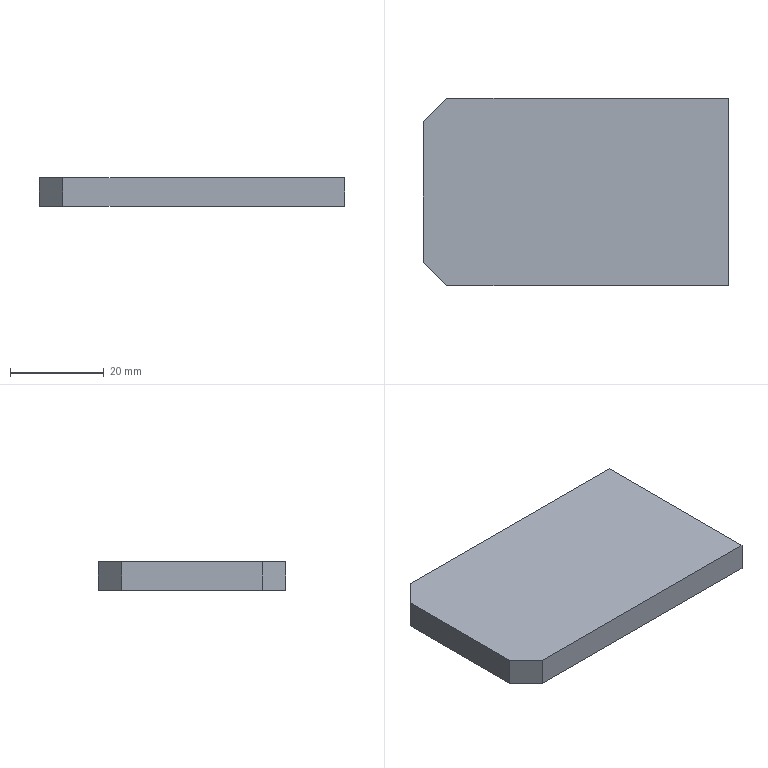Part | STEP file | ASND-0110-Body 1-23 | 1 solid | 8 faces | box 65 x 40 x 6 mm | volume 15450 mm3 | plane 8
STEP:
#1=CARTESIAN_POINT('',(0.,0.,0.));
#2=DIRECTION('',(0.,0.,1.));
#3=DIRECTION('',(1.,0.,0.));
#4=AXIS2_PLACEMENT_3D('',#1,#2,#3);
#5=CARTESIAN_POINT('',(25.,0.,10.));
#6=VERTEX_POINT('',#5);
#7=CARTESIAN_POINT('',(20.,5.,10.));
#8=VERTEX_POINT('',#7);
#9=CARTESIAN_POINT('',(25.,0.,10.));
#10=DIRECTION('',(-0.7071,0.7071,0.));
#11=VECTOR('',#10,1.);
#12=LINE('',#9,#11);
#13=CARTESIAN_POINT('',(22.5,2.5,0.));
#14=DIRECTION('',(-0.7071,-0.7071,0.));
#15=DIRECTION('',(-0.5774,0.5774,0.5774));
#16=AXIS2_PLACEMENT_3D('',#13,#14,#15);
#17=PLANE('',#16);
#18=CARTESIAN_POINT('',(2.887,-10.206));
#19=DIRECTION('',(0.8165,0.5774));
#20=VECTOR('',#19,1.);
#21=LINE('',#18,#20);
#22=(GEOMETRIC_REPRESENTATION_CONTEXT(2)PARAMETRIC_REPRESENTATION_CONTEXT()REPRESENTATION_CONTEXT('',''));
#23=DEFINITIONAL_REPRESENTATION('',(#21),#22);
#24=PCURVE('',#17,#23);
#25=CARTESIAN_POINT('',(65.,20.,10.));
#26=DIRECTION('',(0.,0.,1.));
#27=DIRECTION('',(0.7071,0.7071,0.));
#28=AXIS2_PLACEMENT_3D('',#25,#26,#27);
#29=PLANE('',#28);
#30=CARTESIAN_POINT('',(-42.426,14.142));
#31=DIRECTION('',(0.,1.));
#32=VECTOR('',#31,1.);
#33=LINE('',#30,#32);
#34=(GEOMETRIC_REPRESENTATION_CONTEXT(2)PARAMETRIC_REPRESENTATION_CONTEXT()REPRESENTATION_CONTEXT('',''));
#35=DEFINITIONAL_REPRESENTATION('',(#33),#34);
#36=PCURVE('',#29,#35);
#37=SURFACE_CURVE('',#12,(#24,#36),.PCURVE_S1.);
#38=EDGE_CURVE('',#6,#8,#37,.T.);
#39=ORIENTED_EDGE('',*,*,#38,.T.);
#40=CARTESIAN_POINT('',(20.,5.,4.));
#41=VERTEX_POINT('',#40);
#42=CARTESIAN_POINT('',(20.,5.,10.));
#43=DIRECTION('',(0.,0.,-1.));
#44=VECTOR('',#43,1.);
#45=LINE('',#42,#44);
#46=CARTESIAN_POINT('',(8.66,-6.124));
#47=DIRECTION('',(-0.5774,0.8165));
#48=VECTOR('',#47,1.);
#49=LINE('',#46,#48);
#50=(GEOMETRIC_REPRESENTATION_CONTEXT(2)PARAMETRIC_REPRESENTATION_CONTEXT()REPRESENTATION_CONTEXT('',''));
#51=DEFINITIONAL_REPRESENTATION('',(#49),#50);
#52=PCURVE('',#17,#51);
#53=CARTESIAN_POINT('',(20.,0.,0.));
#54=DIRECTION('',(-1.,0.,0.));
#55=DIRECTION('',(0.,0.7071,0.7071));
#56=AXIS2_PLACEMENT_3D('',#53,#54,#55);
#57=PLANE('',#56);
#58=CARTESIAN_POINT('',(10.607,-3.536));
#59=DIRECTION('',(-0.7071,0.7071));
#60=VECTOR('',#59,1.);
#61=LINE('',#58,#60);
#62=(GEOMETRIC_REPRESENTATION_CONTEXT(2)PARAMETRIC_REPRESENTATION_CONTEXT()REPRESENTATION_CONTEXT('',''));
#63=DEFINITIONAL_REPRESENTATION('',(#61),#62);
#64=PCURVE('',#57,#63);
#65=SURFACE_CURVE('',#45,(#52,#64),.PCURVE_S1.);
#66=EDGE_CURVE('',#8,#41,#65,.T.);
#67=ORIENTED_EDGE('',*,*,#66,.T.);
#68=CARTESIAN_POINT('',(25.,0.,4.));
#69=VERTEX_POINT('',#68);
#70=CARTESIAN_POINT('',(20.,5.,4.));
#71=DIRECTION('',(0.7071,-0.7071,0.));
#72=VECTOR('',#71,1.);
#73=LINE('',#70,#72);
#74=CARTESIAN_POINT('',(5.196,-1.225));
#75=DIRECTION('',(-0.8165,-0.5774));
#76=VECTOR('',#75,1.);
#77=LINE('',#74,#76);
#78=(GEOMETRIC_REPRESENTATION_CONTEXT(2)PARAMETRIC_REPRESENTATION_CONTEXT()REPRESENTATION_CONTEXT('',''));
#79=DEFINITIONAL_REPRESENTATION('',(#77),#78);
#80=PCURVE('',#17,#79);
#81=CARTESIAN_POINT('',(65.,20.,4.));
#82=DIRECTION('',(0.,0.,1.));
#83=DIRECTION('',(0.7071,0.7071,0.));
#84=AXIS2_PLACEMENT_3D('',#81,#82,#83);
#85=PLANE('',#84);
#86=CARTESIAN_POINT('',(-42.426,21.213));
#87=DIRECTION('',(0.,-1.));
#88=VECTOR('',#87,1.);
#89=LINE('',#86,#88);
#90=(GEOMETRIC_REPRESENTATION_CONTEXT(2)PARAMETRIC_REPRESENTATION_CONTEXT()REPRESENTATION_CONTEXT('',''));
#91=DEFINITIONAL_REPRESENTATION('',(#89),#90);
#92=PCURVE('',#85,#91);
#93=SURFACE_CURVE('',#73,(#80,#92),.PCURVE_S1.);
#94=EDGE_CURVE('',#41,#69,#93,.T.);
#95=ORIENTED_EDGE('',*,*,#94,.T.);
#96=CARTESIAN_POINT('',(25.,0.,0.));
#97=DIRECTION('',(0.,0.,1.));
#98=VECTOR('',#97,1.);
#99=LINE('',#96,#98);
#100=CARTESIAN_POINT('',(-2.887,-2.041));
#101=DIRECTION('',(0.5774,-0.8165));
#102=VECTOR('',#101,1.);
#103=LINE('',#100,#102);
#104=(GEOMETRIC_REPRESENTATION_CONTEXT(2)PARAMETRIC_REPRESENTATION_CONTEXT()REPRESENTATION_CONTEXT('',''));
#105=DEFINITIONAL_REPRESENTATION('',(#103),#104);
#106=PCURVE('',#17,#105);
#107=CARTESIAN_POINT('',(130.,0.,0.));
#108=DIRECTION('',(0.,-1.,0.));
#109=DIRECTION('',(0.7071,0.,0.7071));
#110=AXIS2_PLACEMENT_3D('',#107,#108,#109);
#111=PLANE('',#110);
#112=CARTESIAN_POINT('',(-74.246,74.246));
#113=DIRECTION('',(0.7071,0.7071));
#114=VECTOR('',#113,1.);
#115=LINE('',#112,#114);
#116=(GEOMETRIC_REPRESENTATION_CONTEXT(2)PARAMETRIC_REPRESENTATION_CONTEXT()REPRESENTATION_CONTEXT('',''));
#117=DEFINITIONAL_REPRESENTATION('',(#115),#116);
#118=PCURVE('',#111,#117);
#119=SURFACE_CURVE('',#99,(#106,#118),.PCURVE_S1.);
#120=EDGE_CURVE('',#69,#6,#119,.T.);
#121=ORIENTED_EDGE('',*,*,#120,.T.);
#122=EDGE_LOOP('',(#39,#67,#95,#121));
#123=FACE_BOUND('',#122,.T.);
#124=ADVANCED_FACE('',(#123),#17,.T.);
#125=ORIENTED_EDGE('',*,*,#120,.F.);
#126=CARTESIAN_POINT('',(85.,0.,4.));
#127=VERTEX_POINT('',#126);
#128=CARTESIAN_POINT('',(5.,0.,4.));
#129=DIRECTION('',(1.,0.,0.));
#130=VECTOR('',#129,1.);
#131=LINE('',#128,#130);
#132=CARTESIAN_POINT('',(-85.56,91.217));
#133=DIRECTION('',(0.7071,-0.7071));
#134=VECTOR('',#133,1.);
#135=LINE('',#132,#134);
#136=(GEOMETRIC_REPRESENTATION_CONTEXT(2)PARAMETRIC_REPRESENTATION_CONTEXT()REPRESENTATION_CONTEXT('',''));
#137=DEFINITIONAL_REPRESENTATION('',(#135),#136);
#138=PCURVE('',#111,#137);
#139=CARTESIAN_POINT('',(-56.569,28.284));
#140=DIRECTION('',(0.7071,-0.7071));
#141=VECTOR('',#140,1.);
#142=LINE('',#139,#141);
#143=(GEOMETRIC_REPRESENTATION_CONTEXT(2)PARAMETRIC_REPRESENTATION_CONTEXT()REPRESENTATION_CONTEXT('',''));
#144=DEFINITIONAL_REPRESENTATION('',(#142),#143);
#145=PCURVE('',#85,#144);
#146=SURFACE_CURVE('',#131,(#138,#145),.PCURVE_S1.);
#147=EDGE_CURVE('',#69,#127,#146,.T.);
#148=ORIENTED_EDGE('',*,*,#147,.T.);
#149=CARTESIAN_POINT('',(85.,0.,10.));
#150=VERTEX_POINT('',#149);
#151=CARTESIAN_POINT('',(85.,0.,0.));
#152=DIRECTION('',(0.,0.,1.));
#153=VECTOR('',#152,1.);
#154=LINE('',#151,#153);
#155=CARTESIAN_POINT('',(-31.82,31.82));
#156=DIRECTION('',(0.7071,0.7071));
#157=VECTOR('',#156,1.);
#158=LINE('',#155,#157);
#159=(GEOMETRIC_REPRESENTATION_CONTEXT(2)PARAMETRIC_REPRESENTATION_CONTEXT()REPRESENTATION_CONTEXT('',''));
#160=DEFINITIONAL_REPRESENTATION('',(#158),#159);
#161=PCURVE('',#111,#160);
#162=CARTESIAN_POINT('',(85.,40.,0.));
#163=DIRECTION('',(1.,0.,0.));
#164=DIRECTION('',(0.,0.7071,0.7071));
#165=AXIS2_PLACEMENT_3D('',#162,#163,#164);
#166=PLANE('',#165);
#167=CARTESIAN_POINT('',(-28.284,28.284));
#168=DIRECTION('',(0.7071,0.7071));
#169=VECTOR('',#168,1.);
#170=LINE('',#167,#169);
#171=(GEOMETRIC_REPRESENTATION_CONTEXT(2)PARAMETRIC_REPRESENTATION_CONTEXT()REPRESENTATION_CONTEXT('',''));
#172=DEFINITIONAL_REPRESENTATION('',(#170),#171);
#173=PCURVE('',#166,#172);
#174=SURFACE_CURVE('',#154,(#161,#173),.PCURVE_S1.);
#175=EDGE_CURVE('',#127,#150,#174,.T.);
#176=ORIENTED_EDGE('',*,*,#175,.T.);
#177=CARTESIAN_POINT('',(85.,0.,10.));
#178=DIRECTION('',(-1.,0.,0.));
#179=VECTOR('',#178,1.);
#180=LINE('',#177,#179);
#181=CARTESIAN_POINT('',(-24.749,38.891));
#182=DIRECTION('',(-0.7071,0.7071));
#183=VECTOR('',#182,1.);
#184=LINE('',#181,#183);
#185=(GEOMETRIC_REPRESENTATION_CONTEXT(2)PARAMETRIC_REPRESENTATION_CONTEXT()REPRESENTATION_CONTEXT('',''));
#186=DEFINITIONAL_REPRESENTATION('',(#184),#185);
#187=PCURVE('',#111,#186);
#188=CARTESIAN_POINT('',(0.,-28.284));
#189=DIRECTION('',(-0.7071,0.7071));
#190=VECTOR('',#189,1.);
#191=LINE('',#188,#190);
#192=(GEOMETRIC_REPRESENTATION_CONTEXT(2)PARAMETRIC_REPRESENTATION_CONTEXT()REPRESENTATION_CONTEXT('',''));
#193=DEFINITIONAL_REPRESENTATION('',(#191),#192);
#194=PCURVE('',#29,#193);
#195=SURFACE_CURVE('',#180,(#187,#194),.PCURVE_S1.);
#196=EDGE_CURVE('',#150,#6,#195,.T.);
#197=ORIENTED_EDGE('',*,*,#196,.T.);
#198=EDGE_LOOP('',(#125,#148,#176,#197));
#199=FACE_BOUND('',#198,.T.);
#200=ADVANCED_FACE('',(#199),#111,.T.);
#201=ORIENTED_EDGE('',*,*,#94,.F.);
#202=CARTESIAN_POINT('',(20.,35.,4.));
#203=VERTEX_POINT('',#202);
#204=CARTESIAN_POINT('',(20.,35.,4.));
#205=DIRECTION('',(0.,-1.,0.));
#206=VECTOR('',#205,1.);
#207=LINE('',#204,#206);
#208=CARTESIAN_POINT('',(-21.213,42.426));
#209=DIRECTION('',(-0.7071,-0.7071));
#210=VECTOR('',#209,1.);
#211=LINE('',#208,#210);
#212=(GEOMETRIC_REPRESENTATION_CONTEXT(2)PARAMETRIC_REPRESENTATION_CONTEXT()REPRESENTATION_CONTEXT('',''));
#213=DEFINITIONAL_REPRESENTATION('',(#211),#212);
#214=PCURVE('',#85,#213);
#215=CARTESIAN_POINT('',(27.577,21.92));
#216=DIRECTION('',(-0.7071,-0.7071));
#217=VECTOR('',#216,1.);
#218=LINE('',#215,#217);
#219=(GEOMETRIC_REPRESENTATION_CONTEXT(2)PARAMETRIC_REPRESENTATION_CONTEXT()REPRESENTATION_CONTEXT('',''));
#220=DEFINITIONAL_REPRESENTATION('',(#218),#219);
#221=PCURVE('',#57,#220);
#222=SURFACE_CURVE('',#207,(#214,#221),.PCURVE_S1.);
#223=EDGE_CURVE('',#203,#41,#222,.T.);
#224=ORIENTED_EDGE('',*,*,#223,.F.);
#225=CARTESIAN_POINT('',(25.,40.,4.));
#226=VERTEX_POINT('',#225);
#227=CARTESIAN_POINT('',(25.,40.,4.));
#228=DIRECTION('',(-0.7071,-0.7071,0.));
#229=VECTOR('',#228,1.);
#230=LINE('',#227,#229);
#231=CARTESIAN_POINT('',(-14.142,42.426));
#232=DIRECTION('',(-1.,0.));
#233=VECTOR('',#232,1.);
#234=LINE('',#231,#233);
#235=(GEOMETRIC_REPRESENTATION_CONTEXT(2)PARAMETRIC_REPRESENTATION_CONTEXT()REPRESENTATION_CONTEXT('',''));
#236=DEFINITIONAL_REPRESENTATION('',(#234),#235);
#237=PCURVE('',#85,#236);
#238=CARTESIAN_POINT('',(22.5,37.5,0.));
#239=DIRECTION('',(-0.7071,0.7071,0.));
#240=DIRECTION('',(0.5774,0.5774,0.5774));
#241=AXIS2_PLACEMENT_3D('',#238,#239,#240);
#242=PLANE('',#241);
#243=CARTESIAN_POINT('',(5.196,-1.225));
#244=DIRECTION('',(-0.8165,-0.5774));
#245=VECTOR('',#244,1.);
#246=LINE('',#243,#245);
#247=(GEOMETRIC_REPRESENTATION_CONTEXT(2)PARAMETRIC_REPRESENTATION_CONTEXT()REPRESENTATION_CONTEXT('',''));
#248=DEFINITIONAL_REPRESENTATION('',(#246),#247);
#249=PCURVE('',#242,#248);
#250=SURFACE_CURVE('',#230,(#237,#249),.PCURVE_S1.);
#251=EDGE_CURVE('',#226,#203,#250,.T.);
#252=ORIENTED_EDGE('',*,*,#251,.F.);
#253=CARTESIAN_POINT('',(85.,40.,4.));
#254=VERTEX_POINT('',#253);
#255=CARTESIAN_POINT('',(85.,40.,4.));
#256=DIRECTION('',(-1.,0.,0.));
#257=VECTOR('',#256,1.);
#258=LINE('',#255,#257);
#259=CARTESIAN_POINT('',(28.284,0.));
#260=DIRECTION('',(-0.7071,0.7071));
#261=VECTOR('',#260,1.);
#262=LINE('',#259,#261);
#263=(GEOMETRIC_REPRESENTATION_CONTEXT(2)PARAMETRIC_REPRESENTATION_CONTEXT()REPRESENTATION_CONTEXT('',''));
#264=DEFINITIONAL_REPRESENTATION('',(#262),#263);
#265=PCURVE('',#85,#264);
#266=CARTESIAN_POINT('',(0.,40.,0.));
#267=DIRECTION('',(0.,1.,0.));
#268=DIRECTION('',(0.7071,0.,0.7071));
#269=AXIS2_PLACEMENT_3D('',#266,#267,#268);
#270=PLANE('',#269);
#271=CARTESIAN_POINT('',(62.933,57.276));
#272=DIRECTION('',(-0.7071,-0.7071));
#273=VECTOR('',#272,1.);
#274=LINE('',#271,#273);
#275=(GEOMETRIC_REPRESENTATION_CONTEXT(2)PARAMETRIC_REPRESENTATION_CONTEXT()REPRESENTATION_CONTEXT('',''));
#276=DEFINITIONAL_REPRESENTATION('',(#274),#275);
#277=PCURVE('',#270,#276);
#278=SURFACE_CURVE('',#258,(#265,#277),.PCURVE_S1.);
#279=EDGE_CURVE('',#254,#226,#278,.T.);
#280=ORIENTED_EDGE('',*,*,#279,.F.);
#281=CARTESIAN_POINT('',(85.,0.,4.));
#282=DIRECTION('',(0.,1.,0.));
#283=VECTOR('',#282,1.);
#284=LINE('',#281,#283);
#285=CARTESIAN_POINT('',(0.,-28.284));
#286=DIRECTION('',(0.7071,0.7071));
#287=VECTOR('',#286,1.);
#288=LINE('',#285,#287);
#289=(GEOMETRIC_REPRESENTATION_CONTEXT(2)PARAMETRIC_REPRESENTATION_CONTEXT()REPRESENTATION_CONTEXT('',''));
#290=DEFINITIONAL_REPRESENTATION('',(#288),#289);
#291=PCURVE('',#85,#290);
#292=CARTESIAN_POINT('',(-25.456,31.113));
#293=DIRECTION('',(0.7071,-0.7071));
#294=VECTOR('',#293,1.);
#295=LINE('',#292,#294);
#296=(GEOMETRIC_REPRESENTATION_CONTEXT(2)PARAMETRIC_REPRESENTATION_CONTEXT()REPRESENTATION_CONTEXT('',''));
#297=DEFINITIONAL_REPRESENTATION('',(#295),#296);
#298=PCURVE('',#166,#297);
#299=SURFACE_CURVE('',#284,(#291,#298),.PCURVE_S1.);
#300=EDGE_CURVE('',#127,#254,#299,.T.);
#301=ORIENTED_EDGE('',*,*,#300,.F.);
#302=ORIENTED_EDGE('',*,*,#147,.F.);
#303=EDGE_LOOP('',(#201,#224,#252,#280,#301,#302));
#304=FACE_BOUND('',#303,.T.);
#305=ADVANCED_FACE('',(#304),#85,.F.);
#306=CARTESIAN_POINT('',(20.,35.,10.));
#307=VERTEX_POINT('',#306);
#308=CARTESIAN_POINT('',(25.,40.,10.));
#309=VERTEX_POINT('',#308);
#310=CARTESIAN_POINT('',(20.,35.,10.));
#311=DIRECTION('',(0.7071,0.7071,0.));
#312=VECTOR('',#311,1.);
#313=LINE('',#310,#312);
#314=CARTESIAN_POINT('',(2.887,-10.206));
#315=DIRECTION('',(0.8165,0.5774));
#316=VECTOR('',#315,1.);
#317=LINE('',#314,#316);
#318=(GEOMETRIC_REPRESENTATION_CONTEXT(2)PARAMETRIC_REPRESENTATION_CONTEXT()REPRESENTATION_CONTEXT('',''));
#319=DEFINITIONAL_REPRESENTATION('',(#317),#318);
#320=PCURVE('',#242,#319);
#321=CARTESIAN_POINT('',(-21.213,42.426));
#322=DIRECTION('',(1.,0.));
#323=VECTOR('',#322,1.);
#324=LINE('',#321,#323);
#325=(GEOMETRIC_REPRESENTATION_CONTEXT(2)PARAMETRIC_REPRESENTATION_CONTEXT()REPRESENTATION_CONTEXT('',''));
#326=DEFINITIONAL_REPRESENTATION('',(#324),#325);
#327=PCURVE('',#29,#326);
#328=SURFACE_CURVE('',#313,(#320,#327),.PCURVE_S1.);
#329=EDGE_CURVE('',#307,#309,#328,.T.);
#330=ORIENTED_EDGE('',*,*,#329,.T.);
#331=CARTESIAN_POINT('',(25.,40.,10.));
#332=DIRECTION('',(0.,0.,-1.));
#333=VECTOR('',#332,1.);
#334=LINE('',#331,#333);
#335=CARTESIAN_POINT('',(8.66,-6.124));
#336=DIRECTION('',(-0.5774,0.8165));
#337=VECTOR('',#336,1.);
#338=LINE('',#335,#337);
#339=(GEOMETRIC_REPRESENTATION_CONTEXT(2)PARAMETRIC_REPRESENTATION_CONTEXT()REPRESENTATION_CONTEXT('',''));
#340=DEFINITIONAL_REPRESENTATION('',(#338),#339);
#341=PCURVE('',#242,#340);
#342=CARTESIAN_POINT('',(24.749,10.607));
#343=DIRECTION('',(-0.7071,0.7071));
#344=VECTOR('',#343,1.);
#345=LINE('',#342,#344);
#346=(GEOMETRIC_REPRESENTATION_CONTEXT(2)PARAMETRIC_REPRESENTATION_CONTEXT()REPRESENTATION_CONTEXT('',''));
#347=DEFINITIONAL_REPRESENTATION('',(#345),#346);
#348=PCURVE('',#270,#347);
#349=SURFACE_CURVE('',#334,(#341,#348),.PCURVE_S1.);
#350=EDGE_CURVE('',#309,#226,#349,.T.);
#351=ORIENTED_EDGE('',*,*,#350,.T.);
#352=ORIENTED_EDGE('',*,*,#251,.T.);
#353=CARTESIAN_POINT('',(20.,35.,0.));
#354=DIRECTION('',(0.,0.,1.));
#355=VECTOR('',#354,1.);
#356=LINE('',#353,#355);
#357=CARTESIAN_POINT('',(-2.887,-2.041));
#358=DIRECTION('',(0.5774,-0.8165));
#359=VECTOR('',#358,1.);
#360=LINE('',#357,#359);
#361=(GEOMETRIC_REPRESENTATION_CONTEXT(2)PARAMETRIC_REPRESENTATION_CONTEXT()REPRESENTATION_CONTEXT('',''));
#362=DEFINITIONAL_REPRESENTATION('',(#360),#361);
#363=PCURVE('',#242,#362);
#364=CARTESIAN_POINT('',(24.749,24.749));
#365=DIRECTION('',(0.7071,-0.7071));
#366=VECTOR('',#365,1.);
#367=LINE('',#364,#366);
#368=(GEOMETRIC_REPRESENTATION_CONTEXT(2)PARAMETRIC_REPRESENTATION_CONTEXT()REPRESENTATION_CONTEXT('',''));
#369=DEFINITIONAL_REPRESENTATION('',(#367),#368);
#370=PCURVE('',#57,#369);
#371=SURFACE_CURVE('',#356,(#363,#370),.PCURVE_S1.);
#372=EDGE_CURVE('',#203,#307,#371,.T.);
#373=ORIENTED_EDGE('',*,*,#372,.T.);
#374=EDGE_LOOP('',(#330,#351,#352,#373));
#375=FACE_BOUND('',#374,.T.);
#376=ADVANCED_FACE('',(#375),#242,.T.);
#377=ORIENTED_EDGE('',*,*,#350,.F.);
#378=CARTESIAN_POINT('',(85.,40.,10.));
#379=VERTEX_POINT('',#378);
#380=CARTESIAN_POINT('',(5.,40.,10.));
#381=DIRECTION('',(1.,0.,0.));
#382=VECTOR('',#381,1.);
#383=LINE('',#380,#382);
#384=CARTESIAN_POINT('',(10.607,-3.536));
#385=DIRECTION('',(0.7071,0.7071));
#386=VECTOR('',#385,1.);
#387=LINE('',#384,#386);
#388=(GEOMETRIC_REPRESENTATION_CONTEXT(2)PARAMETRIC_REPRESENTATION_CONTEXT()REPRESENTATION_CONTEXT('',''));
#389=DEFINITIONAL_REPRESENTATION('',(#387),#388);
#390=PCURVE('',#270,#389);
#391=CARTESIAN_POINT('',(-28.284,56.569));
#392=DIRECTION('',(0.7071,-0.7071));
#393=VECTOR('',#392,1.);
#394=LINE('',#391,#393);
#395=(GEOMETRIC_REPRESENTATION_CONTEXT(2)PARAMETRIC_REPRESENTATION_CONTEXT()REPRESENTATION_CONTEXT('',''));
#396=DEFINITIONAL_REPRESENTATION('',(#394),#395);
#397=PCURVE('',#29,#396);
#398=SURFACE_CURVE('',#383,(#390,#397),.PCURVE_S1.);
#399=EDGE_CURVE('',#309,#379,#398,.T.);
#400=ORIENTED_EDGE('',*,*,#399,.T.);
#401=CARTESIAN_POINT('',(85.,40.,0.));
#402=DIRECTION('',(0.,0.,1.));
#403=VECTOR('',#402,1.);
#404=LINE('',#401,#403);
#405=CARTESIAN_POINT('',(60.104,60.104));
#406=DIRECTION('',(0.7071,-0.7071));
#407=VECTOR('',#406,1.);
#408=LINE('',#405,#407);
#409=(GEOMETRIC_REPRESENTATION_CONTEXT(2)PARAMETRIC_REPRESENTATION_CONTEXT()REPRESENTATION_CONTEXT('',''));
#410=DEFINITIONAL_REPRESENTATION('',(#408),#409);
#411=PCURVE('',#270,#410);
#412=CARTESIAN_POINT('',(0.,0.));
#413=DIRECTION('',(0.7071,0.7071));
#414=VECTOR('',#413,1.);
#415=LINE('',#412,#414);
#416=(GEOMETRIC_REPRESENTATION_CONTEXT(2)PARAMETRIC_REPRESENTATION_CONTEXT()REPRESENTATION_CONTEXT('',''));
#417=DEFINITIONAL_REPRESENTATION('',(#415),#416);
#418=PCURVE('',#166,#417);
#419=SURFACE_CURVE('',#404,(#411,#418),.PCURVE_S1.);
#420=EDGE_CURVE('',#254,#379,#419,.T.);
#421=ORIENTED_EDGE('',*,*,#420,.F.);
#422=ORIENTED_EDGE('',*,*,#279,.T.);
#423=EDGE_LOOP('',(#377,#400,#421,#422));
#424=FACE_BOUND('',#423,.T.);
#425=ADVANCED_FACE('',(#424),#270,.T.);
#426=ORIENTED_EDGE('',*,*,#66,.F.);
#427=CARTESIAN_POINT('',(20.,5.,10.));
#428=DIRECTION('',(0.,1.,0.));
#429=VECTOR('',#428,1.);
#430=LINE('',#427,#429);
#431=CARTESIAN_POINT('',(10.607,-3.536));
#432=DIRECTION('',(0.7071,0.7071));
#433=VECTOR('',#432,1.);
#434=LINE('',#431,#433);
#435=(GEOMETRIC_REPRESENTATION_CONTEXT(2)PARAMETRIC_REPRESENTATION_CONTEXT()REPRESENTATION_CONTEXT('',''));
#436=DEFINITIONAL_REPRESENTATION('',(#434),#435);
#437=PCURVE('',#57,#436);
#438=CARTESIAN_POINT('',(-42.426,21.213));
#439=DIRECTION('',(0.7071,0.7071));
#440=VECTOR('',#439,1.);
#441=LINE('',#438,#440);
#442=(GEOMETRIC_REPRESENTATION_CONTEXT(2)PARAMETRIC_REPRESENTATION_CONTEXT()REPRESENTATION_CONTEXT('',''));
#443=DEFINITIONAL_REPRESENTATION('',(#441),#442);
#444=PCURVE('',#29,#443);
#445=SURFACE_CURVE('',#430,(#437,#444),.PCURVE_S1.);
#446=EDGE_CURVE('',#8,#307,#445,.T.);
#447=ORIENTED_EDGE('',*,*,#446,.T.);
#448=ORIENTED_EDGE('',*,*,#372,.F.);
#449=ORIENTED_EDGE('',*,*,#223,.T.);
#450=EDGE_LOOP('',(#426,#447,#448,#449));
#451=FACE_BOUND('',#450,.T.);
#452=ADVANCED_FACE('',(#451),#57,.T.);
#453=CARTESIAN_POINT('',(85.,40.,10.));
#454=DIRECTION('',(0.,-1.,0.));
#455=VECTOR('',#454,1.);
#456=LINE('',#453,#455);
#457=CARTESIAN_POINT('',(7.071,7.071));
#458=DIRECTION('',(-0.7071,0.7071));
#459=VECTOR('',#458,1.);
#460=LINE('',#457,#459);
#461=(GEOMETRIC_REPRESENTATION_CONTEXT(2)PARAMETRIC_REPRESENTATION_CONTEXT()REPRESENTATION_CONTEXT('',''));
#462=DEFINITIONAL_REPRESENTATION('',(#460),#461);
#463=PCURVE('',#166,#462);
#464=CARTESIAN_POINT('',(28.284,0.));
#465=DIRECTION('',(-0.7071,-0.7071));
#466=VECTOR('',#465,1.);
#467=LINE('',#464,#466);
#468=(GEOMETRIC_REPRESENTATION_CONTEXT(2)PARAMETRIC_REPRESENTATION_CONTEXT()REPRESENTATION_CONTEXT('',''));
#469=DEFINITIONAL_REPRESENTATION('',(#467),#468);
#470=PCURVE('',#29,#469);
#471=SURFACE_CURVE('',#456,(#463,#470),.PCURVE_S1.);
#472=EDGE_CURVE('',#379,#150,#471,.T.);
#473=ORIENTED_EDGE('',*,*,#472,.T.);
#474=ORIENTED_EDGE('',*,*,#175,.F.);
#475=ORIENTED_EDGE('',*,*,#300,.T.);
#476=ORIENTED_EDGE('',*,*,#420,.T.);
#477=EDGE_LOOP('',(#473,#474,#475,#476));
#478=FACE_BOUND('',#477,.T.);
#479=ADVANCED_FACE('',(#478),#166,.T.);
#480=ORIENTED_EDGE('',*,*,#38,.F.);
#481=ORIENTED_EDGE('',*,*,#196,.F.);
#482=ORIENTED_EDGE('',*,*,#472,.F.);
#483=ORIENTED_EDGE('',*,*,#399,.F.);
#484=ORIENTED_EDGE('',*,*,#329,.F.);
#485=ORIENTED_EDGE('',*,*,#446,.F.);
#486=EDGE_LOOP('',(#480,#481,#482,#483,#484,#485));
#487=FACE_BOUND('',#486,.T.);
#488=ADVANCED_FACE('',(#487),#29,.T.);
#489=CLOSED_SHELL('',(#124,#200,#305,#376,#425,#452,#479,#488));
#490=MANIFOLD_SOLID_BREP('',#489);
#491=(LENGTH_UNIT()NAMED_UNIT(*)SI_UNIT(.MILLI.,.METRE.));
#492=UNCERTAINTY_MEASURE_WITH_UNIT(LENGTH_MEASURE(0.0000001),#491,'','');
#493=(NAMED_UNIT(*)PLANE_ANGLE_UNIT()SI_UNIT($,.RADIAN.));
#494=(NAMED_UNIT(*)SI_UNIT($,.STERADIAN.)SOLID_ANGLE_UNIT());
#495=(GEOMETRIC_REPRESENTATION_CONTEXT(3)GLOBAL_UNCERTAINTY_ASSIGNED_CONTEXT((#492))GLOBAL_UNIT_ASSIGNED_CONTEXT((#491,#493,#494))REPRESENTATION_CONTEXT('',''));
#496=ADVANCED_BREP_SHAPE_REPRESENTATION('',(#4,#490),#495);